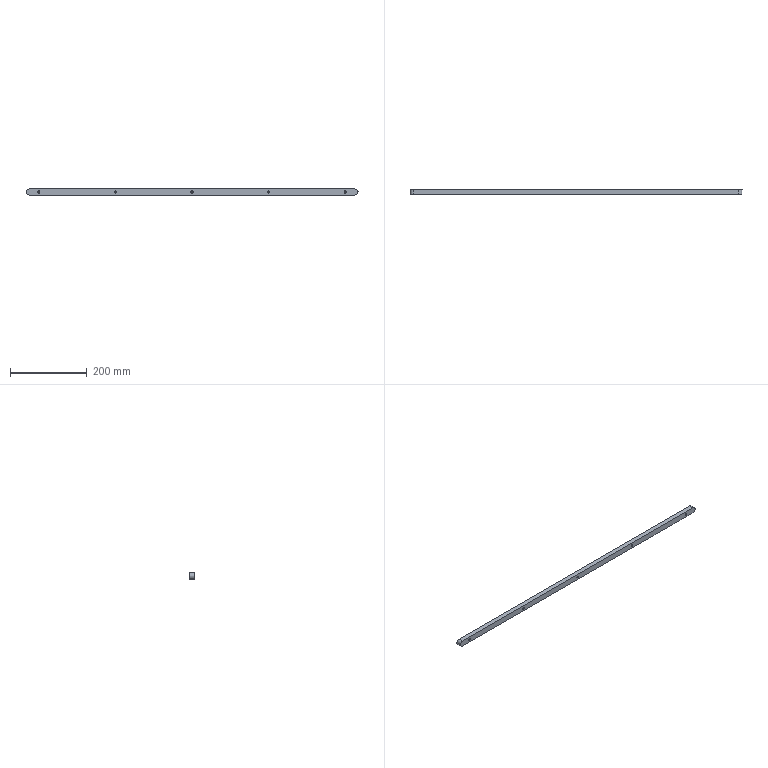Part | STEP file | ROTATION MC_NEW VER-0610_579 | 1 solid | 21 faces | box 867 x 12.8 x 16 mm | volume 173749 mm3 | cylinder 12 | plane 9 | commonest cylinder face diameters 5.5 x5 10 x5 16 x2
STEP:
#1=CARTESIAN_POINT('',(-381.969,304.768,-46.091));
#2=VERTEX_POINT('',#1);
#3=CARTESIAN_POINT('',(-381.969,304.768,-56.091));
#4=VERTEX_POINT('',#3);
#5=CARTESIAN_POINT('',(-381.969,304.768,-51.091));
#6=DIRECTION('',(0.,-1.,0.));
#7=DIRECTION('',(0.,0.,1.));
#8=AXIS2_PLACEMENT_3D('',#5,#6,#7);
#9=CIRCLE('',#8,5.);
#10=EDGE_CURVE('',#2,#4,#9,.T.);
#11=ORIENTED_EDGE('',*,*,#10,.F.);
#12=CARTESIAN_POINT('',(-381.969,304.768,-51.091));
#13=DIRECTION('',(0.,-1.,0.));
#14=DIRECTION('',(0.,0.,1.));
#15=AXIS2_PLACEMENT_3D('',#12,#13,#14);
#16=CIRCLE('',#15,5.);
#17=EDGE_CURVE('',#4,#2,#16,.T.);
#18=ORIENTED_EDGE('',*,*,#17,.F.);
#19=CARTESIAN_POINT('',(-381.969,298.968,-56.091));
#20=VERTEX_POINT('',#19);
#21=CARTESIAN_POINT('',(-381.969,304.768,-56.091));
#22=DIRECTION('',(0.,-1.,0.));
#23=VECTOR('',#22,5.);
#24=LINE('',#21,#23);
#25=EDGE_CURVE('',#4,#20,#24,.T.);
#26=ORIENTED_EDGE('',*,*,#25,.T.);
#27=CARTESIAN_POINT('',(-381.969,298.968,-46.091));
#28=VERTEX_POINT('',#27);
#29=CARTESIAN_POINT('',(-381.969,298.968,-51.091));
#30=DIRECTION('',(0.,1.,0.));
#31=DIRECTION('',(0.,0.,1.));
#32=AXIS2_PLACEMENT_3D('',#29,#30,#31);
#33=CIRCLE('',#32,5.);
#34=EDGE_CURVE('',#28,#20,#33,.T.);
#35=ORIENTED_EDGE('',*,*,#34,.F.);
#36=CARTESIAN_POINT('',(-381.969,298.968,-51.091));
#37=DIRECTION('',(0.,1.,0.));
#38=DIRECTION('',(0.,0.,1.));
#39=AXIS2_PLACEMENT_3D('',#36,#37,#38);
#40=CIRCLE('',#39,5.);
#41=EDGE_CURVE('',#20,#28,#40,.T.);
#42=ORIENTED_EDGE('',*,*,#41,.F.);
#43=ORIENTED_EDGE('',*,*,#25,.F.);
#44=EDGE_LOOP('',(#11,#18,#26,#35,#42,#43));
#45=FACE_OUTER_BOUND('',#44,.T.);
#46=CARTESIAN_POINT('',(-381.969,304.768,-51.091));
#47=DIRECTION('',(0.,-1.,0.));
#48=DIRECTION('',(0.,0.,1.));
#49=AXIS2_PLACEMENT_3D('',#46,#47,#48);
#50=CYLINDRICAL_SURFACE('',#49,5.);
#51=ADVANCED_FACE('',(#45),#50,.F.);
#52=ORIENTED_EDGE('',*,*,#34,.T.);
#53=ORIENTED_EDGE('',*,*,#41,.T.);
#54=EDGE_LOOP('',(#52,#53));
#55=FACE_OUTER_BOUND('',#54,.T.);
#56=CARTESIAN_POINT('',(-381.969,298.968,-48.341));
#57=VERTEX_POINT('',#56);
#58=CARTESIAN_POINT('',(-381.969,298.968,-53.841));
#59=VERTEX_POINT('',#58);
#60=CARTESIAN_POINT('',(-381.969,298.968,-51.091));
#61=DIRECTION('',(0.,1.,0.));
#62=DIRECTION('',(0.,0.,1.));
#63=AXIS2_PLACEMENT_3D('',#60,#61,#62);
#64=CIRCLE('',#63,2.75);
#65=EDGE_CURVE('',#57,#59,#64,.T.);
#66=ORIENTED_EDGE('',*,*,#65,.F.);
#67=CARTESIAN_POINT('',(-381.969,298.968,-51.091));
#68=DIRECTION('',(0.,1.,0.));
#69=DIRECTION('',(0.,0.,1.));
#70=AXIS2_PLACEMENT_3D('',#67,#68,#69);
#71=CIRCLE('',#70,2.75);
#72=EDGE_CURVE('',#59,#57,#71,.T.);
#73=ORIENTED_EDGE('',*,*,#72,.F.);
#74=EDGE_LOOP('',(#66,#73));
#75=FACE_BOUND('',#74,.T.);
#76=CARTESIAN_POINT('',(-381.969,298.968,-51.091));
#77=DIRECTION('',(0.,-1.,0.));
#78=DIRECTION('',(0.,0.,-1.));
#79=AXIS2_PLACEMENT_3D('',#76,#77,#78);
#80=PLANE('',#79);
#81=ADVANCED_FACE('',(#55,#75),#80,.F.);
#82=ORIENTED_EDGE('',*,*,#65,.T.);
#83=CARTESIAN_POINT('',(-381.969,291.968,-53.841));
#84=VERTEX_POINT('',#83);
#85=CARTESIAN_POINT('',(-381.969,284.768,-53.841));
#86=DIRECTION('',(0.,-1.,0.));
#87=VECTOR('',#86,2.75);
#88=LINE('',#85,#87);
#89=EDGE_CURVE('',#59,#84,#88,.T.);
#90=ORIENTED_EDGE('',*,*,#89,.T.);
#91=CARTESIAN_POINT('',(-381.969,291.968,-51.091));
#92=DIRECTION('',(0.,1.,0.));
#93=DIRECTION('',(0.,0.,-1.));
#94=AXIS2_PLACEMENT_3D('',#91,#92,#93);
#95=CIRCLE('',#94,2.75);
#96=EDGE_CURVE('',#84,#84,#95,.T.);
#97=ORIENTED_EDGE('',*,*,#96,.F.);
#98=ORIENTED_EDGE('',*,*,#89,.F.);
#99=ORIENTED_EDGE('',*,*,#72,.T.);
#100=EDGE_LOOP('',(#82,#90,#97,#98,#99));
#101=FACE_OUTER_BOUND('',#100,.T.);
#102=CARTESIAN_POINT('',(-381.969,284.768,-51.091));
#103=DIRECTION('',(0.,-1.,0.));
#104=DIRECTION('',(0.,0.,1.));
#105=AXIS2_PLACEMENT_3D('',#102,#103,#104);
#106=CYLINDRICAL_SURFACE('',#105,2.75);
#107=ADVANCED_FACE('',(#101),#106,.F.);
#108=CARTESIAN_POINT('',(-181.969,304.768,-46.091));
#109=VERTEX_POINT('',#108);
#110=CARTESIAN_POINT('',(-181.969,304.768,-56.091));
#111=VERTEX_POINT('',#110);
#112=CARTESIAN_POINT('',(-181.969,304.768,-51.091));
#113=DIRECTION('',(0.,-1.,0.));
#114=DIRECTION('',(0.,0.,1.));
#115=AXIS2_PLACEMENT_3D('',#112,#113,#114);
#116=CIRCLE('',#115,5.);
#117=EDGE_CURVE('',#109,#111,#116,.T.);
#118=ORIENTED_EDGE('',*,*,#117,.F.);
#119=CARTESIAN_POINT('',(-181.969,304.768,-51.091));
#120=DIRECTION('',(0.,-1.,0.));
#121=DIRECTION('',(0.,0.,1.));
#122=AXIS2_PLACEMENT_3D('',#119,#120,#121);
#123=CIRCLE('',#122,5.);
#124=EDGE_CURVE('',#111,#109,#123,.T.);
#125=ORIENTED_EDGE('',*,*,#124,.F.);
#126=CARTESIAN_POINT('',(-181.969,298.968,-56.091));
#127=VERTEX_POINT('',#126);
#128=CARTESIAN_POINT('',(-181.969,304.768,-56.091));
#129=DIRECTION('',(0.,-1.,0.));
#130=VECTOR('',#129,5.);
#131=LINE('',#128,#130);
#132=EDGE_CURVE('',#111,#127,#131,.T.);
#133=ORIENTED_EDGE('',*,*,#132,.T.);
#134=CARTESIAN_POINT('',(-181.969,298.968,-46.091));
#135=VERTEX_POINT('',#134);
#136=CARTESIAN_POINT('',(-181.969,298.968,-51.091));
#137=DIRECTION('',(0.,1.,0.));
#138=DIRECTION('',(0.,0.,1.));
#139=AXIS2_PLACEMENT_3D('',#136,#137,#138);
#140=CIRCLE('',#139,5.);
#141=EDGE_CURVE('',#135,#127,#140,.T.);
#142=ORIENTED_EDGE('',*,*,#141,.F.);
#143=CARTESIAN_POINT('',(-181.969,298.968,-51.091));
#144=DIRECTION('',(0.,1.,0.));
#145=DIRECTION('',(0.,0.,1.));
#146=AXIS2_PLACEMENT_3D('',#143,#144,#145);
#147=CIRCLE('',#146,5.);
#148=EDGE_CURVE('',#127,#135,#147,.T.);
#149=ORIENTED_EDGE('',*,*,#148,.F.);
#150=ORIENTED_EDGE('',*,*,#132,.F.);
#151=EDGE_LOOP('',(#118,#125,#133,#142,#149,#150));
#152=FACE_OUTER_BOUND('',#151,.T.);
#153=CARTESIAN_POINT('',(-181.969,304.768,-51.091));
#154=DIRECTION('',(0.,-1.,0.));
#155=DIRECTION('',(0.,0.,1.));
#156=AXIS2_PLACEMENT_3D('',#153,#154,#155);
#157=CYLINDRICAL_SURFACE('',#156,5.);
#158=ADVANCED_FACE('',(#152),#157,.F.);
#159=ORIENTED_EDGE('',*,*,#141,.T.);
#160=ORIENTED_EDGE('',*,*,#148,.T.);
#161=EDGE_LOOP('',(#159,#160));
#162=FACE_OUTER_BOUND('',#161,.T.);
#163=CARTESIAN_POINT('',(-181.969,298.968,-48.341));
#164=VERTEX_POINT('',#163);
#165=CARTESIAN_POINT('',(-181.969,298.968,-53.841));
#166=VERTEX_POINT('',#165);
#167=CARTESIAN_POINT('',(-181.969,298.968,-51.091));
#168=DIRECTION('',(0.,1.,0.));
#169=DIRECTION('',(0.,0.,1.));
#170=AXIS2_PLACEMENT_3D('',#167,#168,#169);
#171=CIRCLE('',#170,2.75);
#172=EDGE_CURVE('',#164,#166,#171,.T.);
#173=ORIENTED_EDGE('',*,*,#172,.F.);
#174=CARTESIAN_POINT('',(-181.969,298.968,-51.091));
#175=DIRECTION('',(0.,1.,0.));
#176=DIRECTION('',(0.,0.,1.));
#177=AXIS2_PLACEMENT_3D('',#174,#175,#176);
#178=CIRCLE('',#177,2.75);
#179=EDGE_CURVE('',#166,#164,#178,.T.);
#180=ORIENTED_EDGE('',*,*,#179,.F.);
#181=EDGE_LOOP('',(#173,#180));
#182=FACE_BOUND('',#181,.T.);
#183=CARTESIAN_POINT('',(-181.969,298.968,-51.091));
#184=DIRECTION('',(0.,-1.,0.));
#185=DIRECTION('',(0.,0.,-1.));
#186=AXIS2_PLACEMENT_3D('',#183,#184,#185);
#187=PLANE('',#186);
#188=ADVANCED_FACE('',(#162,#182),#187,.F.);
#189=ORIENTED_EDGE('',*,*,#172,.T.);
#190=CARTESIAN_POINT('',(-181.969,291.968,-53.841));
#191=VERTEX_POINT('',#190);
#192=CARTESIAN_POINT('',(-181.969,284.768,-53.841));
#193=DIRECTION('',(0.,-1.,0.));
#194=VECTOR('',#193,2.75);
#195=LINE('',#192,#194);
#196=EDGE_CURVE('',#166,#191,#195,.T.);
#197=ORIENTED_EDGE('',*,*,#196,.T.);
#198=CARTESIAN_POINT('',(-181.969,291.968,-51.091));
#199=DIRECTION('',(0.,1.,0.));
#200=DIRECTION('',(0.,0.,-1.));
#201=AXIS2_PLACEMENT_3D('',#198,#199,#200);
#202=CIRCLE('',#201,2.75);
#203=EDGE_CURVE('',#191,#191,#202,.T.);
#204=ORIENTED_EDGE('',*,*,#203,.F.);
#205=ORIENTED_EDGE('',*,*,#196,.F.);
#206=ORIENTED_EDGE('',*,*,#179,.T.);
#207=EDGE_LOOP('',(#189,#197,#204,#205,#206));
#208=FACE_OUTER_BOUND('',#207,.T.);
#209=CARTESIAN_POINT('',(-181.969,284.768,-51.091));
#210=DIRECTION('',(0.,-1.,0.));
#211=DIRECTION('',(0.,0.,1.));
#212=AXIS2_PLACEMENT_3D('',#209,#210,#211);
#213=CYLINDRICAL_SURFACE('',#212,2.75);
#214=ADVANCED_FACE('',(#208),#213,.F.);
#215=CARTESIAN_POINT('',(18.031,304.768,-46.091));
#216=VERTEX_POINT('',#215);
#217=CARTESIAN_POINT('',(18.031,304.768,-56.091));
#218=VERTEX_POINT('',#217);
#219=CARTESIAN_POINT('',(18.031,304.768,-51.091));
#220=DIRECTION('',(0.,-1.,0.));
#221=DIRECTION('',(0.,0.,1.));
#222=AXIS2_PLACEMENT_3D('',#219,#220,#221);
#223=CIRCLE('',#222,5.);
#224=EDGE_CURVE('',#216,#218,#223,.T.);
#225=ORIENTED_EDGE('',*,*,#224,.F.);
#226=CARTESIAN_POINT('',(18.031,304.768,-51.091));
#227=DIRECTION('',(0.,-1.,0.));
#228=DIRECTION('',(0.,0.,1.));
#229=AXIS2_PLACEMENT_3D('',#226,#227,#228);
#230=CIRCLE('',#229,5.);
#231=EDGE_CURVE('',#218,#216,#230,.T.);
#232=ORIENTED_EDGE('',*,*,#231,.F.);
#233=CARTESIAN_POINT('',(18.031,298.968,-56.091));
#234=VERTEX_POINT('',#233);
#235=CARTESIAN_POINT('',(18.031,304.768,-56.091));
#236=DIRECTION('',(0.,-1.,0.));
#237=VECTOR('',#236,5.);
#238=LINE('',#235,#237);
#239=EDGE_CURVE('',#218,#234,#238,.T.);
#240=ORIENTED_EDGE('',*,*,#239,.T.);
#241=CARTESIAN_POINT('',(18.031,298.968,-46.091));
#242=VERTEX_POINT('',#241);
#243=CARTESIAN_POINT('',(18.031,298.968,-51.091));
#244=DIRECTION('',(0.,1.,0.));
#245=DIRECTION('',(0.,0.,1.));
#246=AXIS2_PLACEMENT_3D('',#243,#244,#245);
#247=CIRCLE('',#246,5.);
#248=EDGE_CURVE('',#242,#234,#247,.T.);
#249=ORIENTED_EDGE('',*,*,#248,.F.);
#250=CARTESIAN_POINT('',(18.031,298.968,-51.091));
#251=DIRECTION('',(0.,1.,0.));
#252=DIRECTION('',(0.,0.,1.));
#253=AXIS2_PLACEMENT_3D('',#250,#251,#252);
#254=CIRCLE('',#253,5.);
#255=EDGE_CURVE('',#234,#242,#254,.T.);
#256=ORIENTED_EDGE('',*,*,#255,.F.);
#257=ORIENTED_EDGE('',*,*,#239,.F.);
#258=EDGE_LOOP('',(#225,#232,#240,#249,#256,#257));
#259=FACE_OUTER_BOUND('',#258,.T.);
#260=CARTESIAN_POINT('',(18.031,304.768,-51.091));
#261=DIRECTION('',(0.,-1.,0.));
#262=DIRECTION('',(0.,0.,1.));
#263=AXIS2_PLACEMENT_3D('',#260,#261,#262);
#264=CYLINDRICAL_SURFACE('',#263,5.);
#265=ADVANCED_FACE('',(#259),#264,.F.);
#266=ORIENTED_EDGE('',*,*,#248,.T.);
#267=ORIENTED_EDGE('',*,*,#255,.T.);
#268=EDGE_LOOP('',(#266,#267));
#269=FACE_OUTER_BOUND('',#268,.T.);
#270=CARTESIAN_POINT('',(18.031,298.968,-48.341));
#271=VERTEX_POINT('',#270);
#272=CARTESIAN_POINT('',(18.031,298.968,-53.841));
#273=VERTEX_POINT('',#272);
#274=CARTESIAN_POINT('',(18.031,298.968,-51.091));
#275=DIRECTION('',(0.,1.,0.));
#276=DIRECTION('',(0.,0.,1.));
#277=AXIS2_PLACEMENT_3D('',#274,#275,#276);
#278=CIRCLE('',#277,2.75);
#279=EDGE_CURVE('',#271,#273,#278,.T.);
#280=ORIENTED_EDGE('',*,*,#279,.F.);
#281=CARTESIAN_POINT('',(18.031,298.968,-51.091));
#282=DIRECTION('',(0.,1.,0.));
#283=DIRECTION('',(0.,0.,1.));
#284=AXIS2_PLACEMENT_3D('',#281,#282,#283);
#285=CIRCLE('',#284,2.75);
#286=EDGE_CURVE('',#273,#271,#285,.T.);
#287=ORIENTED_EDGE('',*,*,#286,.F.);
#288=EDGE_LOOP('',(#280,#287));
#289=FACE_BOUND('',#288,.T.);
#290=CARTESIAN_POINT('',(18.031,298.968,-51.091));
#291=DIRECTION('',(0.,-1.,0.));
#292=DIRECTION('',(0.,0.,-1.));
#293=AXIS2_PLACEMENT_3D('',#290,#291,#292);
#294=PLANE('',#293);
#295=ADVANCED_FACE('',(#269,#289),#294,.F.);
#296=ORIENTED_EDGE('',*,*,#279,.T.);
#297=CARTESIAN_POINT('',(18.031,291.968,-53.841));
#298=VERTEX_POINT('',#297);
#299=CARTESIAN_POINT('',(18.031,284.768,-53.841));
#300=DIRECTION('',(0.,-1.,0.));
#301=VECTOR('',#300,2.75);
#302=LINE('',#299,#301);
#303=EDGE_CURVE('',#273,#298,#302,.T.);
#304=ORIENTED_EDGE('',*,*,#303,.T.);
#305=CARTESIAN_POINT('',(18.031,291.968,-51.091));
#306=DIRECTION('',(0.,1.,0.));
#307=DIRECTION('',(0.,0.,-1.));
#308=AXIS2_PLACEMENT_3D('',#305,#306,#307);
#309=CIRCLE('',#308,2.75);
#310=EDGE_CURVE('',#298,#298,#309,.T.);
#311=ORIENTED_EDGE('',*,*,#310,.F.);
#312=ORIENTED_EDGE('',*,*,#303,.F.);
#313=ORIENTED_EDGE('',*,*,#286,.T.);
#314=EDGE_LOOP('',(#296,#304,#311,#312,#313));
#315=FACE_OUTER_BOUND('',#314,.T.);
#316=CARTESIAN_POINT('',(18.031,284.768,-51.091));
#317=DIRECTION('',(0.,-1.,0.));
#318=DIRECTION('',(0.,0.,1.));
#319=AXIS2_PLACEMENT_3D('',#316,#317,#318);
#320=CYLINDRICAL_SURFACE('',#319,2.75);
#321=ADVANCED_FACE('',(#315),#320,.F.);
#322=CARTESIAN_POINT('',(218.031,304.768,-46.091));
#323=VERTEX_POINT('',#322);
#324=CARTESIAN_POINT('',(218.031,304.768,-56.091));
#325=VERTEX_POINT('',#324);
#326=CARTESIAN_POINT('',(218.031,304.768,-51.091));
#327=DIRECTION('',(0.,-1.,0.));
#328=DIRECTION('',(0.,0.,1.));
#329=AXIS2_PLACEMENT_3D('',#326,#327,#328);
#330=CIRCLE('',#329,5.);
#331=EDGE_CURVE('',#323,#325,#330,.T.);
#332=ORIENTED_EDGE('',*,*,#331,.F.);
#333=CARTESIAN_POINT('',(218.031,304.768,-51.091));
#334=DIRECTION('',(0.,-1.,0.));
#335=DIRECTION('',(0.,0.,1.));
#336=AXIS2_PLACEMENT_3D('',#333,#334,#335);
#337=CIRCLE('',#336,5.);
#338=EDGE_CURVE('',#325,#323,#337,.T.);
#339=ORIENTED_EDGE('',*,*,#338,.F.);
#340=CARTESIAN_POINT('',(218.031,298.968,-56.091));
#341=VERTEX_POINT('',#340);
#342=CARTESIAN_POINT('',(218.031,304.768,-56.091));
#343=DIRECTION('',(0.,-1.,0.));
#344=VECTOR('',#343,5.);
#345=LINE('',#342,#344);
#346=EDGE_CURVE('',#325,#341,#345,.T.);
#347=ORIENTED_EDGE('',*,*,#346,.T.);
#348=CARTESIAN_POINT('',(218.031,298.968,-46.091));
#349=VERTEX_POINT('',#348);
#350=CARTESIAN_POINT('',(218.031,298.968,-51.091));
#351=DIRECTION('',(0.,1.,0.));
#352=DIRECTION('',(0.,0.,1.));
#353=AXIS2_PLACEMENT_3D('',#350,#351,#352);
#354=CIRCLE('',#353,5.);
#355=EDGE_CURVE('',#349,#341,#354,.T.);
#356=ORIENTED_EDGE('',*,*,#355,.F.);
#357=CARTESIAN_POINT('',(218.031,298.968,-51.091));
#358=DIRECTION('',(0.,1.,0.));
#359=DIRECTION('',(0.,0.,1.));
#360=AXIS2_PLACEMENT_3D('',#357,#358,#359);
#361=CIRCLE('',#360,5.);
#362=EDGE_CURVE('',#341,#349,#361,.T.);
#363=ORIENTED_EDGE('',*,*,#362,.F.);
#364=ORIENTED_EDGE('',*,*,#346,.F.);
#365=EDGE_LOOP('',(#332,#339,#347,#356,#363,#364));
#366=FACE_OUTER_BOUND('',#365,.T.);
#367=CARTESIAN_POINT('',(218.031,304.768,-51.091));
#368=DIRECTION('',(0.,-1.,0.));
#369=DIRECTION('',(0.,0.,1.));
#370=AXIS2_PLACEMENT_3D('',#367,#368,#369);
#371=CYLINDRICAL_SURFACE('',#370,5.);
#372=ADVANCED_FACE('',(#366),#371,.F.);
#373=ORIENTED_EDGE('',*,*,#355,.T.);
#374=ORIENTED_EDGE('',*,*,#362,.T.);
#375=EDGE_LOOP('',(#373,#374));
#376=FACE_OUTER_BOUND('',#375,.T.);
#377=CARTESIAN_POINT('',(218.031,298.968,-48.341));
#378=VERTEX_POINT('',#377);
#379=CARTESIAN_POINT('',(218.031,298.968,-53.841));
#380=VERTEX_POINT('',#379);
#381=CARTESIAN_POINT('',(218.031,298.968,-51.091));
#382=DIRECTION('',(0.,1.,0.));
#383=DIRECTION('',(0.,0.,1.));
#384=AXIS2_PLACEMENT_3D('',#381,#382,#383);
#385=CIRCLE('',#384,2.75);
#386=EDGE_CURVE('',#378,#380,#385,.T.);
#387=ORIENTED_EDGE('',*,*,#386,.F.);
#388=CARTESIAN_POINT('',(218.031,298.968,-51.091));
#389=DIRECTION('',(0.,1.,0.));
#390=DIRECTION('',(0.,0.,1.));
#391=AXIS2_PLACEMENT_3D('',#388,#389,#390);
#392=CIRCLE('',#391,2.75);
#393=EDGE_CURVE('',#380,#378,#392,.T.);
#394=ORIENTED_EDGE('',*,*,#393,.F.);
#395=EDGE_LOOP('',(#387,#394));
#396=FACE_BOUND('',#395,.T.);
#397=CARTESIAN_POINT('',(218.031,298.968,-51.091));
#398=DIRECTION('',(0.,-1.,0.));
#399=DIRECTION('',(0.,0.,-1.));
#400=AXIS2_PLACEMENT_3D('',#397,#398,#399);
#401=PLANE('',#400);
#402=ADVANCED_FACE('',(#376,#396),#401,.F.);
#403=ORIENTED_EDGE('',*,*,#386,.T.);
#404=CARTESIAN_POINT('',(218.031,291.968,-53.841));
#405=VERTEX_POINT('',#404);
#406=CARTESIAN_POINT('',(218.031,284.768,-53.841));
#407=DIRECTION('',(0.,-1.,0.));
#408=VECTOR('',#407,2.75);
#409=LINE('',#406,#408);
#410=EDGE_CURVE('',#380,#405,#409,.T.);
#411=ORIENTED_EDGE('',*,*,#410,.T.);
#412=CARTESIAN_POINT('',(218.031,291.968,-51.091));
#413=DIRECTION('',(0.,1.,0.));
#414=DIRECTION('',(0.,0.,-1.));
#415=AXIS2_PLACEMENT_3D('',#412,#413,#414);
#416=CIRCLE('',#415,2.75);
#417=EDGE_CURVE('',#405,#405,#416,.T.);
#418=ORIENTED_EDGE('',*,*,#417,.F.);
#419=ORIENTED_EDGE('',*,*,#410,.F.);
#420=ORIENTED_EDGE('',*,*,#393,.T.);
#421=EDGE_LOOP('',(#403,#411,#418,#419,#420));
#422=FACE_OUTER_BOUND('',#421,.T.);
#423=CARTESIAN_POINT('',(218.031,284.768,-51.091));
#424=DIRECTION('',(0.,-1.,0.));
#425=DIRECTION('',(0.,0.,1.));
#426=AXIS2_PLACEMENT_3D('',#423,#424,#425);
#427=CYLINDRICAL_SURFACE('',#426,2.75);
#428=ADVANCED_FACE('',(#422),#427,.F.);
#429=CARTESIAN_POINT('',(418.031,304.768,-46.091));
#430=VERTEX_POINT('',#429);
#431=CARTESIAN_POINT('',(418.031,304.768,-56.091));
#432=VERTEX_POINT('',#431);
#433=CARTESIAN_POINT('',(418.031,304.768,-51.091));
#434=DIRECTION('',(0.,-1.,0.));
#435=DIRECTION('',(0.,0.,1.));
#436=AXIS2_PLACEMENT_3D('',#433,#434,#435);
#437=CIRCLE('',#436,5.);
#438=EDGE_CURVE('',#430,#432,#437,.T.);
#439=ORIENTED_EDGE('',*,*,#438,.F.);
#440=CARTESIAN_POINT('',(418.031,304.768,-51.091));
#441=DIRECTION('',(0.,-1.,0.));
#442=DIRECTION('',(0.,0.,1.));
#443=AXIS2_PLACEMENT_3D('',#440,#441,#442);
#444=CIRCLE('',#443,5.);
#445=EDGE_CURVE('',#432,#430,#444,.T.);
#446=ORIENTED_EDGE('',*,*,#445,.F.);
#447=CARTESIAN_POINT('',(418.031,298.968,-56.091));
#448=VERTEX_POINT('',#447);
#449=CARTESIAN_POINT('',(418.031,304.768,-56.091));
#450=DIRECTION('',(0.,-1.,0.));
#451=VECTOR('',#450,5.);
#452=LINE('',#449,#451);
#453=EDGE_CURVE('',#432,#448,#452,.T.);
#454=ORIENTED_EDGE('',*,*,#453,.T.);
#455=CARTESIAN_POINT('',(418.031,298.968,-46.091));
#456=VERTEX_POINT('',#455);
#457=CARTESIAN_POINT('',(418.031,298.968,-51.091));
#458=DIRECTION('',(0.,1.,0.));
#459=DIRECTION('',(0.,0.,1.));
#460=AXIS2_PLACEMENT_3D('',#457,#458,#459);
#461=CIRCLE('',#460,5.);
#462=EDGE_CURVE('',#456,#448,#461,.T.);
#463=ORIENTED_EDGE('',*,*,#462,.F.);
#464=CARTESIAN_POINT('',(418.031,298.968,-51.091));
#465=DIRECTION('',(0.,1.,0.));
#466=DIRECTION('',(0.,0.,1.));
#467=AXIS2_PLACEMENT_3D('',#464,#465,#466);
#468=CIRCLE('',#467,5.);
#469=EDGE_CURVE('',#448,#456,#468,.T.);
#470=ORIENTED_EDGE('',*,*,#469,.F.);
#471=ORIENTED_EDGE('',*,*,#453,.F.);
#472=EDGE_LOOP('',(#439,#446,#454,#463,#470,#471));
#473=FACE_OUTER_BOUND('',#472,.T.);
#474=CARTESIAN_POINT('',(418.031,304.768,-51.091));
#475=DIRECTION('',(0.,-1.,0.));
#476=DIRECTION('',(0.,0.,1.));
#477=AXIS2_PLACEMENT_3D('',#474,#475,#476);
#478=CYLINDRICAL_SURFACE('',#477,5.);
#479=ADVANCED_FACE('',(#473),#478,.F.);
#480=ORIENTED_EDGE('',*,*,#462,.T.);
#481=ORIENTED_EDGE('',*,*,#469,.T.);
#482=EDGE_LOOP('',(#480,#481));
#483=FACE_OUTER_BOUND('',#482,.T.);
#484=CARTESIAN_POINT('',(418.031,298.968,-48.341));
#485=VERTEX_POINT('',#484);
#486=CARTESIAN_POINT('',(418.031,298.968,-53.841));
#487=VERTEX_POINT('',#486);
#488=CARTESIAN_POINT('',(418.031,298.968,-51.091));
#489=DIRECTION('',(0.,1.,0.));
#490=DIRECTION('',(0.,0.,1.));
#491=AXIS2_PLACEMENT_3D('',#488,#489,#490);
#492=CIRCLE('',#491,2.75);
#493=EDGE_CURVE('',#485,#487,#492,.T.);
#494=ORIENTED_EDGE('',*,*,#493,.F.);
#495=CARTESIAN_POINT('',(418.031,298.968,-51.091));
#496=DIRECTION('',(0.,1.,0.));
#497=DIRECTION('',(0.,0.,1.));
#498=AXIS2_PLACEMENT_3D('',#495,#496,#497);
#499=CIRCLE('',#498,2.75);
#500=EDGE_CURVE('',#487,#485,#499,.T.);
#501=ORIENTED_EDGE('',*,*,#500,.F.);
#502=EDGE_LOOP('',(#494,#501));
#503=FACE_BOUND('',#502,.T.);
#504=CARTESIAN_POINT('',(418.031,298.968,-51.091));
#505=DIRECTION('',(0.,-1.,0.));
#506=DIRECTION('',(0.,0.,-1.));
#507=AXIS2_PLACEMENT_3D('',#504,#505,#506);
#508=PLANE('',#507);
#509=ADVANCED_FACE('',(#483,#503),#508,.F.);
#510=ORIENTED_EDGE('',*,*,#493,.T.);
#511=CARTESIAN_POINT('',(418.031,291.968,-53.841));
#512=VERTEX_POINT('',#511);
#513=CARTESIAN_POINT('',(418.031,284.768,-53.841));
#514=DIRECTION('',(0.,-1.,0.));
#515=VECTOR('',#514,2.75);
#516=LINE('',#513,#515);
#517=EDGE_CURVE('',#487,#512,#516,.T.);
#518=ORIENTED_EDGE('',*,*,#517,.T.);
#519=CARTESIAN_POINT('',(418.031,291.968,-51.091));
#520=DIRECTION('',(0.,1.,0.));
#521=DIRECTION('',(0.,0.,-1.));
#522=AXIS2_PLACEMENT_3D('',#519,#520,#521);
#523=CIRCLE('',#522,2.75);
#524=EDGE_CURVE('',#512,#512,#523,.T.);
#525=ORIENTED_EDGE('',*,*,#524,.F.);
#526=ORIENTED_EDGE('',*,*,#517,.F.);
#527=ORIENTED_EDGE('',*,*,#500,.T.);
#528=EDGE_LOOP('',(#510,#518,#525,#526,#527));
#529=FACE_OUTER_BOUND('',#528,.T.);
#530=CARTESIAN_POINT('',(418.031,284.768,-51.091));
#531=DIRECTION('',(0.,-1.,0.));
#532=DIRECTION('',(0.,0.,1.));
#533=AXIS2_PLACEMENT_3D('',#530,#531,#532);
#534=CYLINDRICAL_SURFACE('',#533,2.75);
#535=ADVANCED_FACE('',(#529),#534,.F.);
#536=CARTESIAN_POINT('',(-407.469,291.968,-43.091));
#537=VERTEX_POINT('',#536);
#538=CARTESIAN_POINT('',(-407.469,291.968,-59.091));
#539=VERTEX_POINT('',#538);
#540=CARTESIAN_POINT('',(-407.469,291.968,-51.091));
#541=DIRECTION('',(0.,-1.,0.));
#542=DIRECTION('',(0.,0.,1.));
#543=AXIS2_PLACEMENT_3D('',#540,#541,#542);
#544=CIRCLE('',#543,8.);
#545=EDGE_CURVE('',#537,#539,#544,.T.);
#546=ORIENTED_EDGE('',*,*,#545,.T.);
#547=CARTESIAN_POINT('',(443.531,291.968,-59.091));
#548=VERTEX_POINT('',#547);
#549=CARTESIAN_POINT('',(-407.469,291.968,-59.091));
#550=DIRECTION('',(1.,0.,0.));
#551=VECTOR('',#550,851.);
#552=LINE('',#549,#551);
#553=EDGE_CURVE('',#539,#548,#552,.T.);
#554=ORIENTED_EDGE('',*,*,#553,.T.);
#555=CARTESIAN_POINT('',(443.531,291.968,-43.091));
#556=VERTEX_POINT('',#555);
#557=CARTESIAN_POINT('',(443.531,291.968,-51.091));
#558=DIRECTION('',(0.,-1.,0.));
#559=DIRECTION('',(0.,0.,-1.));
#560=AXIS2_PLACEMENT_3D('',#557,#558,#559);
#561=CIRCLE('',#560,8.);
#562=EDGE_CURVE('',#548,#556,#561,.T.);
#563=ORIENTED_EDGE('',*,*,#562,.T.);
#564=CARTESIAN_POINT('',(443.531,291.968,-43.091));
#565=DIRECTION('',(-1.,0.,0.));
#566=VECTOR('',#565,851.);
#567=LINE('',#564,#566);
#568=EDGE_CURVE('',#556,#537,#567,.T.);
#569=ORIENTED_EDGE('',*,*,#568,.T.);
#570=EDGE_LOOP('',(#546,#554,#563,#569));
#571=FACE_OUTER_BOUND('',#570,.T.);
#572=ORIENTED_EDGE('',*,*,#524,.T.);
#573=EDGE_LOOP('',(#572));
#574=FACE_BOUND('',#573,.T.);
#575=ORIENTED_EDGE('',*,*,#417,.T.);
#576=EDGE_LOOP('',(#575));
#577=FACE_BOUND('',#576,.T.);
#578=ORIENTED_EDGE('',*,*,#310,.T.);
#579=EDGE_LOOP('',(#578));
#580=FACE_BOUND('',#579,.T.);
#581=ORIENTED_EDGE('',*,*,#203,.T.);
#582=EDGE_LOOP('',(#581));
#583=FACE_BOUND('',#582,.T.);
#584=ORIENTED_EDGE('',*,*,#96,.T.);
#585=EDGE_LOOP('',(#584));
#586=FACE_BOUND('',#585,.T.);
#587=CARTESIAN_POINT('',(465.871,291.968,-36.591));
#588=DIRECTION('',(0.,1.,0.));
#589=DIRECTION('',(0.,0.,1.));
#590=AXIS2_PLACEMENT_3D('',#587,#588,#589);
#591=PLANE('',#590);
#592=ADVANCED_FACE('',(#571,#574,#577,#580,#583,#586),#591,.F.);
#593=CARTESIAN_POINT('',(-407.469,304.768,-59.091));
#594=VERTEX_POINT('',#593);
#595=CARTESIAN_POINT('',(-407.469,304.768,-43.091));
#596=VERTEX_POINT('',#595);
#597=CARTESIAN_POINT('',(-407.469,304.768,-51.091));
#598=DIRECTION('',(0.,1.,0.));
#599=DIRECTION('',(0.,0.,-1.));
#600=AXIS2_PLACEMENT_3D('',#597,#598,#599);
#601=CIRCLE('',#600,8.);
#602=EDGE_CURVE('',#594,#596,#601,.T.);
#603=ORIENTED_EDGE('',*,*,#602,.F.);
#604=CARTESIAN_POINT('',(-407.469,304.768,-59.091));
#605=DIRECTION('',(0.,-1.,0.));
#606=VECTOR('',#605,15.8);
#607=LINE('',#604,#606);
#608=EDGE_CURVE('',#594,#539,#607,.T.);
#609=ORIENTED_EDGE('',*,*,#608,.T.);
#610=ORIENTED_EDGE('',*,*,#545,.F.);
#611=CARTESIAN_POINT('',(-407.469,288.968,-43.091));
#612=DIRECTION('',(0.,1.,0.));
#613=VECTOR('',#612,15.8);
#614=LINE('',#611,#613);
#615=EDGE_CURVE('',#537,#596,#614,.T.);
#616=ORIENTED_EDGE('',*,*,#615,.T.);
#617=EDGE_LOOP('',(#603,#609,#610,#616));
#618=FACE_OUTER_BOUND('',#617,.T.);
#619=CARTESIAN_POINT('',(-407.469,288.968,-51.091));
#620=DIRECTION('',(0.,1.,0.));
#621=DIRECTION('',(0.,0.,1.));
#622=AXIS2_PLACEMENT_3D('',#619,#620,#621);
#623=CYLINDRICAL_SURFACE('',#622,8.);
#624=ADVANCED_FACE('',(#618),#623,.T.);
#625=ORIENTED_EDGE('',*,*,#602,.T.);
#626=CARTESIAN_POINT('',(443.531,304.768,-43.091));
#627=VERTEX_POINT('',#626);
#628=CARTESIAN_POINT('',(-407.469,304.768,-43.091));
#629=DIRECTION('',(1.,0.,0.));
#630=VECTOR('',#629,851.);
#631=LINE('',#628,#630);
#632=EDGE_CURVE('',#596,#627,#631,.T.);
#633=ORIENTED_EDGE('',*,*,#632,.T.);
#634=CARTESIAN_POINT('',(443.531,304.768,-59.091));
#635=VERTEX_POINT('',#634);
#636=CARTESIAN_POINT('',(443.531,304.768,-51.091));
#637=DIRECTION('',(0.,1.,0.));
#638=DIRECTION('',(0.,0.,1.));
#639=AXIS2_PLACEMENT_3D('',#636,#637,#638);
#640=CIRCLE('',#639,8.);
#641=EDGE_CURVE('',#627,#635,#640,.T.);
#642=ORIENTED_EDGE('',*,*,#641,.T.);
#643=CARTESIAN_POINT('',(443.531,304.768,-59.091));
#644=DIRECTION('',(-1.,0.,0.));
#645=VECTOR('',#644,851.);
#646=LINE('',#643,#645);
#647=EDGE_CURVE('',#635,#594,#646,.T.);
#648=ORIENTED_EDGE('',*,*,#647,.T.);
#649=EDGE_LOOP('',(#625,#633,#642,#648));
#650=FACE_OUTER_BOUND('',#649,.T.);
#651=ORIENTED_EDGE('',*,*,#438,.T.);
#652=ORIENTED_EDGE('',*,*,#445,.T.);
#653=EDGE_LOOP('',(#651,#652));
#654=FACE_BOUND('',#653,.T.);
#655=ORIENTED_EDGE('',*,*,#331,.T.);
#656=ORIENTED_EDGE('',*,*,#338,.T.);
#657=EDGE_LOOP('',(#655,#656));
#658=FACE_BOUND('',#657,.T.);
#659=ORIENTED_EDGE('',*,*,#224,.T.);
#660=ORIENTED_EDGE('',*,*,#231,.T.);
#661=EDGE_LOOP('',(#659,#660));
#662=FACE_BOUND('',#661,.T.);
#663=ORIENTED_EDGE('',*,*,#117,.T.);
#664=ORIENTED_EDGE('',*,*,#124,.T.);
#665=EDGE_LOOP('',(#663,#664));
#666=FACE_BOUND('',#665,.T.);
#667=ORIENTED_EDGE('',*,*,#10,.T.);
#668=ORIENTED_EDGE('',*,*,#17,.T.);
#669=EDGE_LOOP('',(#667,#668));
#670=FACE_BOUND('',#669,.T.);
#671=CARTESIAN_POINT('',(465.871,304.768,-34.591));
#672=DIRECTION('',(0.,-1.,0.));
#673=DIRECTION('',(0.,0.,-1.));
#674=AXIS2_PLACEMENT_3D('',#671,#672,#673);
#675=PLANE('',#674);
#676=ADVANCED_FACE('',(#650,#654,#658,#662,#666,#670),#675,.F.);
#677=ORIENTED_EDGE('',*,*,#608,.F.);
#678=ORIENTED_EDGE('',*,*,#647,.F.);
#679=CARTESIAN_POINT('',(443.531,288.968,-59.091));
#680=DIRECTION('',(0.,1.,0.));
#681=VECTOR('',#680,15.8);
#682=LINE('',#679,#681);
#683=EDGE_CURVE('',#548,#635,#682,.T.);
#684=ORIENTED_EDGE('',*,*,#683,.F.);
#685=ORIENTED_EDGE('',*,*,#553,.F.);
#686=EDGE_LOOP('',(#677,#678,#684,#685));
#687=FACE_OUTER_BOUND('',#686,.T.);
#688=CARTESIAN_POINT('',(465.871,362.768,-59.091));
#689=DIRECTION('',(0.,0.,1.));
#690=DIRECTION('',(1.,0.,0.));
#691=AXIS2_PLACEMENT_3D('',#688,#689,#690);
#692=PLANE('',#691);
#693=ADVANCED_FACE('',(#687),#692,.F.);
#694=ORIENTED_EDGE('',*,*,#562,.F.);
#695=ORIENTED_EDGE('',*,*,#683,.T.);
#696=ORIENTED_EDGE('',*,*,#641,.F.);
#697=CARTESIAN_POINT('',(443.531,304.768,-43.091));
#698=DIRECTION('',(0.,-1.,0.));
#699=VECTOR('',#698,15.8);
#700=LINE('',#697,#699);
#701=EDGE_CURVE('',#627,#556,#700,.T.);
#702=ORIENTED_EDGE('',*,*,#701,.T.);
#703=EDGE_LOOP('',(#694,#695,#696,#702));
#704=FACE_OUTER_BOUND('',#703,.T.);
#705=CARTESIAN_POINT('',(443.531,304.768,-51.091));
#706=DIRECTION('',(0.,1.,0.));
#707=DIRECTION('',(0.,0.,1.));
#708=AXIS2_PLACEMENT_3D('',#705,#706,#707);
#709=CYLINDRICAL_SURFACE('',#708,8.);
#710=ADVANCED_FACE('',(#704),#709,.T.);
#711=ORIENTED_EDGE('',*,*,#615,.F.);
#712=ORIENTED_EDGE('',*,*,#568,.F.);
#713=ORIENTED_EDGE('',*,*,#701,.F.);
#714=ORIENTED_EDGE('',*,*,#632,.F.);
#715=EDGE_LOOP('',(#711,#712,#713,#714));
#716=FACE_OUTER_BOUND('',#715,.T.);
#717=CARTESIAN_POINT('',(465.871,362.768,-43.091));
#718=DIRECTION('',(0.,0.,-1.));
#719=DIRECTION('',(-1.,0.,0.));
#720=AXIS2_PLACEMENT_3D('',#717,#718,#719);
#721=PLANE('',#720);
#722=ADVANCED_FACE('',(#716),#721,.F.);
#723=CLOSED_SHELL('',(#51,#81,#107,#158,#188,#214,#265,#295,#321,#372,#402,#428,#479,#509,#535,#592,#624,#676,#693,#710,#722));
#724=MANIFOLD_SOLID_BREP('',#723);
#725=(LENGTH_UNIT()NAMED_UNIT(*)SI_UNIT(.MILLI.,.METRE.));
#726=UNCERTAINTY_MEASURE_WITH_UNIT(LENGTH_MEASURE(0.01),#725,'','');
#727=(NAMED_UNIT(*)PLANE_ANGLE_UNIT()SI_UNIT($,.RADIAN.));
#728=(NAMED_UNIT(*)SI_UNIT($,.STERADIAN.)SOLID_ANGLE_UNIT());
#729=(GEOMETRIC_REPRESENTATION_CONTEXT(3)GLOBAL_UNCERTAINTY_ASSIGNED_CONTEXT((#726))GLOBAL_UNIT_ASSIGNED_CONTEXT((#725,#727,#728))REPRESENTATION_CONTEXT('',''));
#730=ADVANCED_BREP_SHAPE_REPRESENTATION('',(#724),#729);